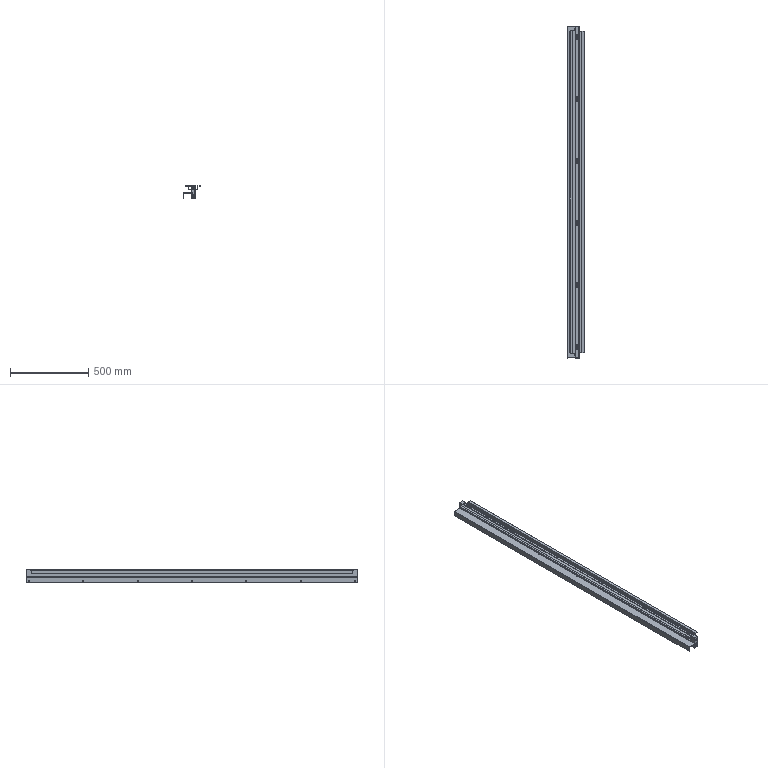Part | SolidWorks | 8 solids | 540 faces | box 110.7 x 2116 x 80 mm | volume 1351065 mm3 | plane 308 | cylinder 232 | commonest cylinder face diameters 6 x116 6.2 x28 9 x18 10 x12 2 x11 3.4 x10